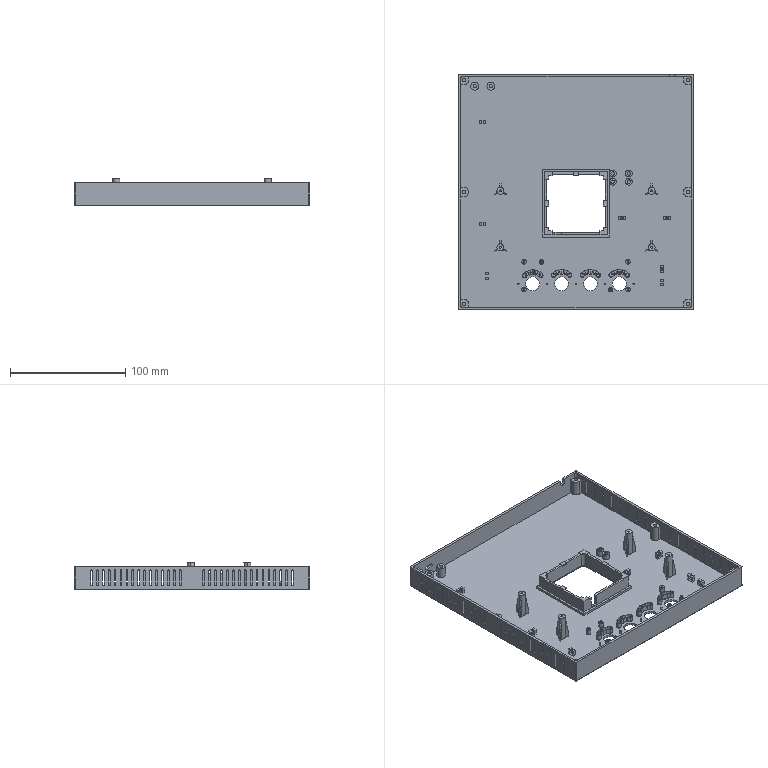Part | SolidWorks | features ICE 31, Fillet 5, Chamfer 3, Extrusion 1, MirrorPattern 1, Shell 1 | 1 solid | 922 faces | box 204 x 204 x 24 mm | volume 118665 mm3 | plane 535 | cylinder 379 | cone 4 | torus 4 | commonest cylinder face diameters 1.5 x144 3 x38 1 x32 1.2 x32 4 x24 6 x16